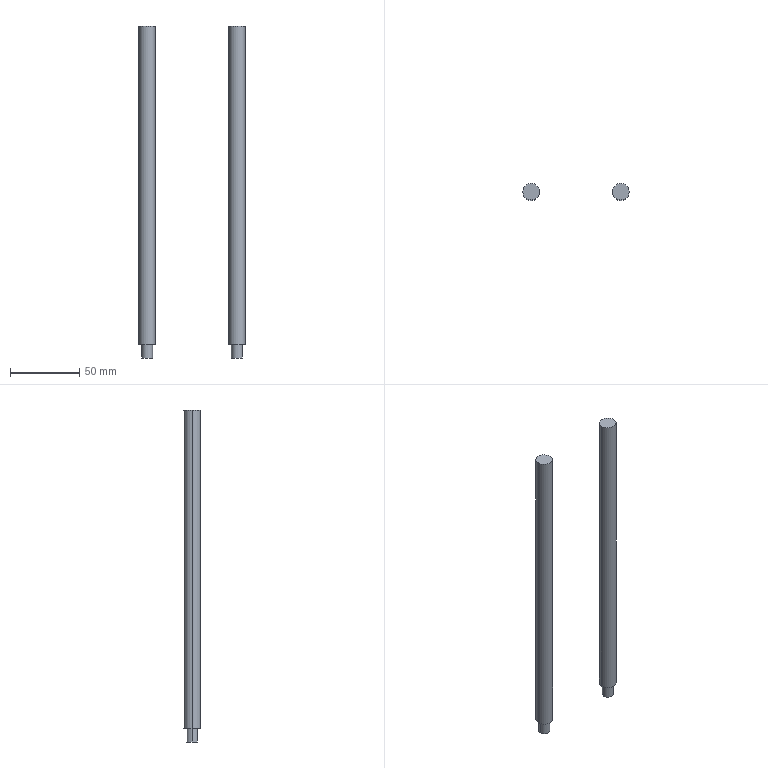Part | STEP file | Part 7^出料机械手-2 | 2 solids | 14 faces | box 77 x 12 x 240.3 mm | volume 53098 mm3 | cylinder 8 | plane 6 | commonest cylinder face diameters 8 x4 12 x4
STEP:
#1=CARTESIAN_POINT('',(23.5,0.,230.3));
#2=VERTEX_POINT('',#1);
#3=CARTESIAN_POINT('',(11.5,0.,230.3));
#4=VERTEX_POINT('',#3);
#5=CARTESIAN_POINT('',(17.5,0.,230.3));
#6=DIRECTION('',(0.,0.,1.));
#7=DIRECTION('',(1.,0.,0.));
#8=AXIS2_PLACEMENT_3D('',#5,#6,#7);
#9=CIRCLE('',#8,6.);
#10=EDGE_CURVE('',#2,#4,#9,.T.);
#11=ORIENTED_EDGE('',*,*,#10,.F.);
#12=CARTESIAN_POINT('',(23.5,0.,0.));
#13=VERTEX_POINT('',#12);
#14=CARTESIAN_POINT('',(23.5,0.,230.3));
#15=DIRECTION('',(0.,0.,-1.));
#16=VECTOR('',#15,1000.);
#17=LINE('',#14,#16);
#18=EDGE_CURVE('',#2,#13,#17,.T.);
#19=ORIENTED_EDGE('',*,*,#18,.T.);
#20=CARTESIAN_POINT('',(11.5,0.,0.));
#21=VERTEX_POINT('',#20);
#22=CARTESIAN_POINT('',(17.5,0.,0.));
#23=DIRECTION('',(0.,0.,1.));
#24=DIRECTION('',(1.,0.,0.));
#25=AXIS2_PLACEMENT_3D('',#22,#23,#24);
#26=CIRCLE('',#25,6.);
#27=EDGE_CURVE('',#13,#21,#26,.T.);
#28=ORIENTED_EDGE('',*,*,#27,.T.);
#29=CARTESIAN_POINT('',(11.5,0.,230.3));
#30=DIRECTION('',(0.,0.,-1.));
#31=VECTOR('',#30,1000.);
#32=LINE('',#29,#31);
#33=EDGE_CURVE('',#4,#21,#32,.T.);
#34=ORIENTED_EDGE('',*,*,#33,.F.);
#35=EDGE_LOOP('',(#11,#19,#28,#34));
#36=FACE_OUTER_BOUND('',#35,.T.);
#37=CARTESIAN_POINT('',(17.5,0.,230.3));
#38=DIRECTION('',(0.,0.,-1.));
#39=DIRECTION('',(-1.,0.,0.));
#40=AXIS2_PLACEMENT_3D('',#37,#38,#39);
#41=CYLINDRICAL_SURFACE('',#40,6.);
#42=ADVANCED_FACE('',(#36),#41,.T.);
#43=CARTESIAN_POINT('',(21.5,0.,-10.));
#44=VERTEX_POINT('',#43);
#45=CARTESIAN_POINT('',(13.5,0.,-10.));
#46=VERTEX_POINT('',#45);
#47=CARTESIAN_POINT('',(17.5,0.,-10.));
#48=DIRECTION('',(0.,0.,1.));
#49=DIRECTION('',(1.,0.,0.));
#50=AXIS2_PLACEMENT_3D('',#47,#48,#49);
#51=CIRCLE('',#50,4.);
#52=EDGE_CURVE('',#44,#46,#51,.T.);
#53=ORIENTED_EDGE('',*,*,#52,.T.);
#54=CARTESIAN_POINT('',(13.5,0.,0.));
#55=VERTEX_POINT('',#54);
#56=CARTESIAN_POINT('',(13.5,0.,-10.));
#57=DIRECTION('',(0.,0.,1.));
#58=VECTOR('',#57,1000.);
#59=LINE('',#56,#58);
#60=EDGE_CURVE('',#46,#55,#59,.T.);
#61=ORIENTED_EDGE('',*,*,#60,.T.);
#62=CARTESIAN_POINT('',(21.5,0.,0.));
#63=VERTEX_POINT('',#62);
#64=CARTESIAN_POINT('',(17.5,0.,0.));
#65=DIRECTION('',(0.,0.,1.));
#66=DIRECTION('',(1.,0.,0.));
#67=AXIS2_PLACEMENT_3D('',#64,#65,#66);
#68=CIRCLE('',#67,4.);
#69=EDGE_CURVE('',#63,#55,#68,.T.);
#70=ORIENTED_EDGE('',*,*,#69,.F.);
#71=CARTESIAN_POINT('',(21.5,0.,-10.));
#72=DIRECTION('',(0.,0.,1.));
#73=VECTOR('',#72,1000.);
#74=LINE('',#71,#73);
#75=EDGE_CURVE('',#44,#63,#74,.T.);
#76=ORIENTED_EDGE('',*,*,#75,.F.);
#77=EDGE_LOOP('',(#53,#61,#70,#76));
#78=FACE_OUTER_BOUND('',#77,.T.);
#79=CARTESIAN_POINT('',(17.5,0.,-10.));
#80=DIRECTION('',(0.,0.,1.));
#81=DIRECTION('',(1.,0.,0.));
#82=AXIS2_PLACEMENT_3D('',#79,#80,#81);
#83=CYLINDRICAL_SURFACE('',#82,4.);
#84=ADVANCED_FACE('',(#78),#83,.T.);
#85=ORIENTED_EDGE('',*,*,#60,.F.);
#86=CARTESIAN_POINT('',(17.5,0.,-10.));
#87=DIRECTION('',(0.,0.,1.));
#88=DIRECTION('',(1.,0.,0.));
#89=AXIS2_PLACEMENT_3D('',#86,#87,#88);
#90=CIRCLE('',#89,4.);
#91=EDGE_CURVE('',#46,#44,#90,.T.);
#92=ORIENTED_EDGE('',*,*,#91,.T.);
#93=ORIENTED_EDGE('',*,*,#75,.T.);
#94=CARTESIAN_POINT('',(17.5,0.,0.));
#95=DIRECTION('',(0.,0.,1.));
#96=DIRECTION('',(1.,0.,0.));
#97=AXIS2_PLACEMENT_3D('',#94,#95,#96);
#98=CIRCLE('',#97,4.);
#99=EDGE_CURVE('',#55,#63,#98,.T.);
#100=ORIENTED_EDGE('',*,*,#99,.F.);
#101=EDGE_LOOP('',(#85,#92,#93,#100));
#102=FACE_OUTER_BOUND('',#101,.T.);
#103=CARTESIAN_POINT('',(17.5,0.,-10.));
#104=DIRECTION('',(0.,0.,1.));
#105=DIRECTION('',(1.,0.,0.));
#106=AXIS2_PLACEMENT_3D('',#103,#104,#105);
#107=CYLINDRICAL_SURFACE('',#106,4.);
#108=ADVANCED_FACE('',(#102),#107,.T.);
#109=ORIENTED_EDGE('',*,*,#52,.F.);
#110=ORIENTED_EDGE('',*,*,#91,.F.);
#111=EDGE_LOOP('',(#109,#110));
#112=FACE_OUTER_BOUND('',#111,.T.);
#113=CARTESIAN_POINT('',(17.5,0.,-10.));
#114=DIRECTION('',(0.,0.,1.));
#115=DIRECTION('',(1.,0.,0.));
#116=AXIS2_PLACEMENT_3D('',#113,#114,#115);
#117=PLANE('',#116);
#118=ADVANCED_FACE('',(#112),#117,.F.);
#119=ORIENTED_EDGE('',*,*,#18,.F.);
#120=CARTESIAN_POINT('',(17.5,0.,230.3));
#121=DIRECTION('',(0.,0.,1.));
#122=DIRECTION('',(1.,0.,0.));
#123=AXIS2_PLACEMENT_3D('',#120,#121,#122);
#124=CIRCLE('',#123,6.);
#125=EDGE_CURVE('',#4,#2,#124,.T.);
#126=ORIENTED_EDGE('',*,*,#125,.F.);
#127=ORIENTED_EDGE('',*,*,#33,.T.);
#128=CARTESIAN_POINT('',(17.5,0.,0.));
#129=DIRECTION('',(0.,0.,1.));
#130=DIRECTION('',(1.,0.,0.));
#131=AXIS2_PLACEMENT_3D('',#128,#129,#130);
#132=CIRCLE('',#131,6.);
#133=EDGE_CURVE('',#21,#13,#132,.T.);
#134=ORIENTED_EDGE('',*,*,#133,.T.);
#135=EDGE_LOOP('',(#119,#126,#127,#134));
#136=FACE_OUTER_BOUND('',#135,.T.);
#137=CARTESIAN_POINT('',(17.5,0.,230.3));
#138=DIRECTION('',(0.,0.,-1.));
#139=DIRECTION('',(-1.,0.,0.));
#140=AXIS2_PLACEMENT_3D('',#137,#138,#139);
#141=CYLINDRICAL_SURFACE('',#140,6.);
#142=ADVANCED_FACE('',(#136),#141,.T.);
#143=ORIENTED_EDGE('',*,*,#125,.T.);
#144=ORIENTED_EDGE('',*,*,#10,.T.);
#145=EDGE_LOOP('',(#143,#144));
#146=FACE_OUTER_BOUND('',#145,.T.);
#147=CARTESIAN_POINT('',(17.5,0.,230.3));
#148=DIRECTION('',(0.,0.,1.));
#149=DIRECTION('',(1.,0.,0.));
#150=AXIS2_PLACEMENT_3D('',#147,#148,#149);
#151=PLANE('',#150);
#152=ADVANCED_FACE('',(#146),#151,.T.);
#153=ORIENTED_EDGE('',*,*,#69,.T.);
#154=ORIENTED_EDGE('',*,*,#99,.T.);
#155=EDGE_LOOP('',(#153,#154));
#156=FACE_BOUND('',#155,.T.);
#157=ORIENTED_EDGE('',*,*,#133,.F.);
#158=ORIENTED_EDGE('',*,*,#27,.F.);
#159=EDGE_LOOP('',(#157,#158));
#160=FACE_OUTER_BOUND('',#159,.T.);
#161=CARTESIAN_POINT('',(17.5,0.,0.));
#162=DIRECTION('',(0.,0.,1.));
#163=DIRECTION('',(1.,0.,0.));
#164=AXIS2_PLACEMENT_3D('',#161,#162,#163);
#165=PLANE('',#164);
#166=ADVANCED_FACE('',(#156,#160),#165,.F.);
#167=CLOSED_SHELL('',(#42,#84,#108,#118,#142,#152,#166));
#168=MANIFOLD_SOLID_BREP('',#167);
#169=CARTESIAN_POINT('',(88.5,0.,230.3));
#170=VERTEX_POINT('',#169);
#171=CARTESIAN_POINT('',(76.5,0.,230.3));
#172=VERTEX_POINT('',#171);
#173=CARTESIAN_POINT('',(82.5,0.,230.3));
#174=DIRECTION('',(0.,0.,1.));
#175=DIRECTION('',(1.,0.,0.));
#176=AXIS2_PLACEMENT_3D('',#173,#174,#175);
#177=CIRCLE('',#176,6.);
#178=EDGE_CURVE('',#170,#172,#177,.T.);
#179=ORIENTED_EDGE('',*,*,#178,.F.);
#180=CARTESIAN_POINT('',(88.5,0.,0.));
#181=VERTEX_POINT('',#180);
#182=CARTESIAN_POINT('',(88.5,0.,230.3));
#183=DIRECTION('',(0.,0.,-1.));
#184=VECTOR('',#183,1000.);
#185=LINE('',#182,#184);
#186=EDGE_CURVE('',#170,#181,#185,.T.);
#187=ORIENTED_EDGE('',*,*,#186,.T.);
#188=CARTESIAN_POINT('',(76.5,0.,0.));
#189=VERTEX_POINT('',#188);
#190=CARTESIAN_POINT('',(82.5,0.,0.));
#191=DIRECTION('',(0.,0.,1.));
#192=DIRECTION('',(1.,0.,0.));
#193=AXIS2_PLACEMENT_3D('',#190,#191,#192);
#194=CIRCLE('',#193,6.);
#195=EDGE_CURVE('',#181,#189,#194,.T.);
#196=ORIENTED_EDGE('',*,*,#195,.T.);
#197=CARTESIAN_POINT('',(76.5,0.,230.3));
#198=DIRECTION('',(0.,0.,-1.));
#199=VECTOR('',#198,1000.);
#200=LINE('',#197,#199);
#201=EDGE_CURVE('',#172,#189,#200,.T.);
#202=ORIENTED_EDGE('',*,*,#201,.F.);
#203=EDGE_LOOP('',(#179,#187,#196,#202));
#204=FACE_OUTER_BOUND('',#203,.T.);
#205=CARTESIAN_POINT('',(82.5,0.,230.3));
#206=DIRECTION('',(0.,0.,-1.));
#207=DIRECTION('',(-1.,0.,0.));
#208=AXIS2_PLACEMENT_3D('',#205,#206,#207);
#209=CYLINDRICAL_SURFACE('',#208,6.);
#210=ADVANCED_FACE('',(#204),#209,.T.);
#211=CARTESIAN_POINT('',(86.5,0.,-10.));
#212=VERTEX_POINT('',#211);
#213=CARTESIAN_POINT('',(78.5,0.,-10.));
#214=VERTEX_POINT('',#213);
#215=CARTESIAN_POINT('',(82.5,0.,-10.));
#216=DIRECTION('',(0.,0.,1.));
#217=DIRECTION('',(1.,0.,0.));
#218=AXIS2_PLACEMENT_3D('',#215,#216,#217);
#219=CIRCLE('',#218,4.);
#220=EDGE_CURVE('',#212,#214,#219,.T.);
#221=ORIENTED_EDGE('',*,*,#220,.T.);
#222=CARTESIAN_POINT('',(78.5,0.,0.));
#223=VERTEX_POINT('',#222);
#224=CARTESIAN_POINT('',(78.5,0.,-10.));
#225=DIRECTION('',(0.,0.,1.));
#226=VECTOR('',#225,1000.);
#227=LINE('',#224,#226);
#228=EDGE_CURVE('',#214,#223,#227,.T.);
#229=ORIENTED_EDGE('',*,*,#228,.T.);
#230=CARTESIAN_POINT('',(86.5,0.,0.));
#231=VERTEX_POINT('',#230);
#232=CARTESIAN_POINT('',(82.5,0.,0.));
#233=DIRECTION('',(0.,0.,1.));
#234=DIRECTION('',(1.,0.,0.));
#235=AXIS2_PLACEMENT_3D('',#232,#233,#234);
#236=CIRCLE('',#235,4.);
#237=EDGE_CURVE('',#231,#223,#236,.T.);
#238=ORIENTED_EDGE('',*,*,#237,.F.);
#239=CARTESIAN_POINT('',(86.5,0.,-10.));
#240=DIRECTION('',(0.,0.,1.));
#241=VECTOR('',#240,1000.);
#242=LINE('',#239,#241);
#243=EDGE_CURVE('',#212,#231,#242,.T.);
#244=ORIENTED_EDGE('',*,*,#243,.F.);
#245=EDGE_LOOP('',(#221,#229,#238,#244));
#246=FACE_OUTER_BOUND('',#245,.T.);
#247=CARTESIAN_POINT('',(82.5,0.,-10.));
#248=DIRECTION('',(0.,0.,1.));
#249=DIRECTION('',(1.,0.,0.));
#250=AXIS2_PLACEMENT_3D('',#247,#248,#249);
#251=CYLINDRICAL_SURFACE('',#250,4.);
#252=ADVANCED_FACE('',(#246),#251,.T.);
#253=ORIENTED_EDGE('',*,*,#228,.F.);
#254=CARTESIAN_POINT('',(82.5,0.,-10.));
#255=DIRECTION('',(0.,0.,1.));
#256=DIRECTION('',(1.,0.,0.));
#257=AXIS2_PLACEMENT_3D('',#254,#255,#256);
#258=CIRCLE('',#257,4.);
#259=EDGE_CURVE('',#214,#212,#258,.T.);
#260=ORIENTED_EDGE('',*,*,#259,.T.);
#261=ORIENTED_EDGE('',*,*,#243,.T.);
#262=CARTESIAN_POINT('',(82.5,0.,0.));
#263=DIRECTION('',(0.,0.,1.));
#264=DIRECTION('',(1.,0.,0.));
#265=AXIS2_PLACEMENT_3D('',#262,#263,#264);
#266=CIRCLE('',#265,4.);
#267=EDGE_CURVE('',#223,#231,#266,.T.);
#268=ORIENTED_EDGE('',*,*,#267,.F.);
#269=EDGE_LOOP('',(#253,#260,#261,#268));
#270=FACE_OUTER_BOUND('',#269,.T.);
#271=CARTESIAN_POINT('',(82.5,0.,-10.));
#272=DIRECTION('',(0.,0.,1.));
#273=DIRECTION('',(1.,0.,0.));
#274=AXIS2_PLACEMENT_3D('',#271,#272,#273);
#275=CYLINDRICAL_SURFACE('',#274,4.);
#276=ADVANCED_FACE('',(#270),#275,.T.);
#277=ORIENTED_EDGE('',*,*,#220,.F.);
#278=ORIENTED_EDGE('',*,*,#259,.F.);
#279=EDGE_LOOP('',(#277,#278));
#280=FACE_OUTER_BOUND('',#279,.T.);
#281=CARTESIAN_POINT('',(82.5,0.,-10.));
#282=DIRECTION('',(0.,0.,1.));
#283=DIRECTION('',(1.,0.,0.));
#284=AXIS2_PLACEMENT_3D('',#281,#282,#283);
#285=PLANE('',#284);
#286=ADVANCED_FACE('',(#280),#285,.F.);
#287=ORIENTED_EDGE('',*,*,#186,.F.);
#288=CARTESIAN_POINT('',(82.5,0.,230.3));
#289=DIRECTION('',(0.,0.,1.));
#290=DIRECTION('',(1.,0.,0.));
#291=AXIS2_PLACEMENT_3D('',#288,#289,#290);
#292=CIRCLE('',#291,6.);
#293=EDGE_CURVE('',#172,#170,#292,.T.);
#294=ORIENTED_EDGE('',*,*,#293,.F.);
#295=ORIENTED_EDGE('',*,*,#201,.T.);
#296=CARTESIAN_POINT('',(82.5,0.,0.));
#297=DIRECTION('',(0.,0.,1.));
#298=DIRECTION('',(1.,0.,0.));
#299=AXIS2_PLACEMENT_3D('',#296,#297,#298);
#300=CIRCLE('',#299,6.);
#301=EDGE_CURVE('',#189,#181,#300,.T.);
#302=ORIENTED_EDGE('',*,*,#301,.T.);
#303=EDGE_LOOP('',(#287,#294,#295,#302));
#304=FACE_OUTER_BOUND('',#303,.T.);
#305=CARTESIAN_POINT('',(82.5,0.,230.3));
#306=DIRECTION('',(0.,0.,-1.));
#307=DIRECTION('',(-1.,0.,0.));
#308=AXIS2_PLACEMENT_3D('',#305,#306,#307);
#309=CYLINDRICAL_SURFACE('',#308,6.);
#310=ADVANCED_FACE('',(#304),#309,.T.);
#311=ORIENTED_EDGE('',*,*,#293,.T.);
#312=ORIENTED_EDGE('',*,*,#178,.T.);
#313=EDGE_LOOP('',(#311,#312));
#314=FACE_OUTER_BOUND('',#313,.T.);
#315=CARTESIAN_POINT('',(82.5,0.,230.3));
#316=DIRECTION('',(0.,0.,1.));
#317=DIRECTION('',(1.,0.,0.));
#318=AXIS2_PLACEMENT_3D('',#315,#316,#317);
#319=PLANE('',#318);
#320=ADVANCED_FACE('',(#314),#319,.T.);
#321=ORIENTED_EDGE('',*,*,#237,.T.);
#322=ORIENTED_EDGE('',*,*,#267,.T.);
#323=EDGE_LOOP('',(#321,#322));
#324=FACE_BOUND('',#323,.T.);
#325=ORIENTED_EDGE('',*,*,#301,.F.);
#326=ORIENTED_EDGE('',*,*,#195,.F.);
#327=EDGE_LOOP('',(#325,#326));
#328=FACE_OUTER_BOUND('',#327,.T.);
#329=CARTESIAN_POINT('',(82.5,0.,0.));
#330=DIRECTION('',(0.,0.,1.));
#331=DIRECTION('',(1.,0.,0.));
#332=AXIS2_PLACEMENT_3D('',#329,#330,#331);
#333=PLANE('',#332);
#334=ADVANCED_FACE('',(#324,#328),#333,.F.);
#335=CLOSED_SHELL('',(#210,#252,#276,#286,#310,#320,#334));
#336=MANIFOLD_SOLID_BREP('',#335);
#337=CARTESIAN_POINT('',(0.,0.,0.));
#338=DIRECTION('',(0.,0.,1.));
#339=DIRECTION('',(1.,0.,0.));
#340=AXIS2_PLACEMENT_3D('',#337,#338,#339);
#341=(LENGTH_UNIT()NAMED_UNIT(*)SI_UNIT(.MILLI.,.METRE.));
#342=UNCERTAINTY_MEASURE_WITH_UNIT(LENGTH_MEASURE(0.00001),#341,'','');
#343=(NAMED_UNIT(*)PLANE_ANGLE_UNIT()SI_UNIT($,.RADIAN.));
#344=(NAMED_UNIT(*)SI_UNIT($,.STERADIAN.)SOLID_ANGLE_UNIT());
#345=(GEOMETRIC_REPRESENTATION_CONTEXT(3)GLOBAL_UNCERTAINTY_ASSIGNED_CONTEXT((#342))GLOBAL_UNIT_ASSIGNED_CONTEXT((#341,#343,#344))REPRESENTATION_CONTEXT('',''));
#346=ADVANCED_BREP_SHAPE_REPRESENTATION('',(#168,#336,#340),#345);